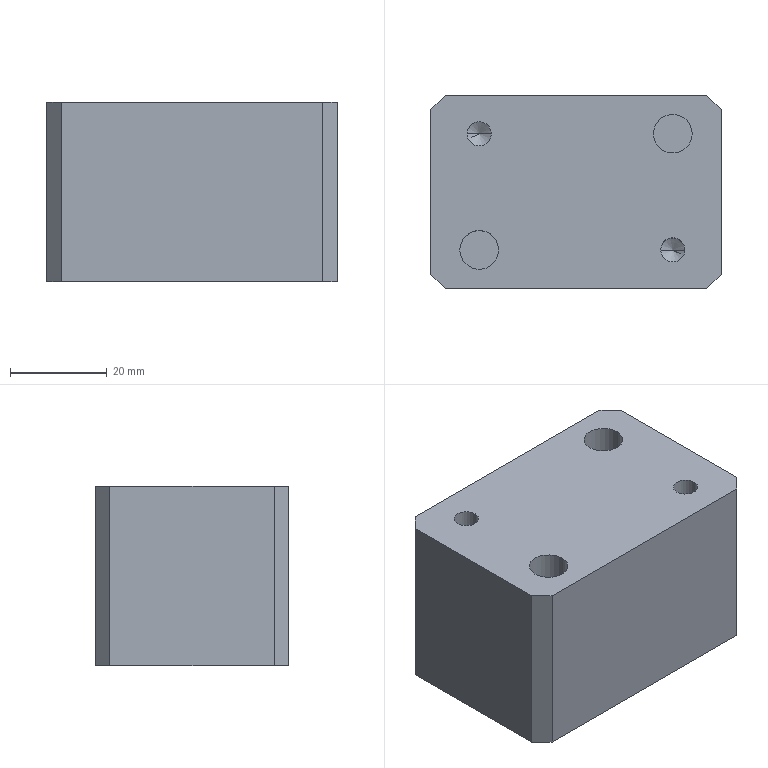Part | SolidWorks | features HoleWzd 4, Chamfer 1, Extrusion 1 | 1 solid | 42 faces | box 60 x 40 x 37 mm | volume 85137 mm3 | cylinder 16 | plane 14 | cone 12 | commonest cylinder face diameters 5 x8 8 x8
STEP:
#1=CARTESIAN_POINT('',(17.998,42.192,0.525));
#2=VERTEX_POINT('',#1);
#3=CARTESIAN_POINT('',(12.998,42.192,0.525));
#4=VERTEX_POINT('',#3);
#5=CARTESIAN_POINT('',(15.498,42.192,0.525));
#6=DIRECTION('',(0.,0.,-1.));
#7=DIRECTION('',(-1.,0.,0.));
#8=AXIS2_PLACEMENT_3D('',#5,#6,#7);
#9=CIRCLE('',#8,2.5);
#10=EDGE_CURVE('',#2,#4,#9,.T.);
#11=ORIENTED_EDGE('',*,*,#10,.F.);
#12=CARTESIAN_POINT('',(18.523,42.192,0.));
#13=VERTEX_POINT('',#12);
#14=CARTESIAN_POINT('',(18.523,42.192,0.));
#15=DIRECTION('',(0.7071,0.,-0.7071));
#16=VECTOR('',#15,1000.);
#17=LINE('',#14,#16);
#18=EDGE_CURVE('',#2,#13,#17,.T.);
#19=ORIENTED_EDGE('',*,*,#18,.T.);
#20=CARTESIAN_POINT('',(12.473,42.192,0.));
#21=VERTEX_POINT('',#20);
#22=CARTESIAN_POINT('',(15.498,42.192,0.));
#23=DIRECTION('',(0.,0.,-1.));
#24=DIRECTION('',(-1.,0.,0.));
#25=AXIS2_PLACEMENT_3D('',#22,#23,#24);
#26=CIRCLE('',#25,3.025);
#27=EDGE_CURVE('',#13,#21,#26,.T.);
#28=ORIENTED_EDGE('',*,*,#27,.T.);
#29=CARTESIAN_POINT('',(12.473,42.192,0.));
#30=DIRECTION('',(-0.7071,0.,-0.7071));
#31=VECTOR('',#30,1000.);
#32=LINE('',#29,#31);
#33=EDGE_CURVE('',#4,#21,#32,.T.);
#34=ORIENTED_EDGE('',*,*,#33,.F.);
#35=EDGE_LOOP('',(#11,#19,#28,#34));
#36=FACE_OUTER_BOUND('',#35,.T.);
#37=CARTESIAN_POINT('',(15.498,42.192,0.));
#38=DIRECTION('',(0.,0.,-1.));
#39=DIRECTION('',(-1.,0.,0.));
#40=AXIS2_PLACEMENT_3D('',#37,#38,#39);
#41=CONICAL_SURFACE('',#40,3.025,0.7854);
#42=ADVANCED_FACE('',(#36),#41,.F.);
#43=CARTESIAN_POINT('',(17.998,42.192,12.));
#44=VERTEX_POINT('',#43);
#45=CARTESIAN_POINT('',(12.998,42.192,12.));
#46=VERTEX_POINT('',#45);
#47=CARTESIAN_POINT('',(15.498,42.192,12.));
#48=DIRECTION('',(0.,0.,-1.));
#49=DIRECTION('',(-1.,0.,0.));
#50=AXIS2_PLACEMENT_3D('',#47,#48,#49);
#51=CIRCLE('',#50,2.5);
#52=EDGE_CURVE('',#44,#46,#51,.T.);
#53=ORIENTED_EDGE('',*,*,#52,.F.);
#54=CARTESIAN_POINT('',(17.998,42.192,0.));
#55=DIRECTION('',(0.,0.,-1.));
#56=VECTOR('',#55,1000.);
#57=LINE('',#54,#56);
#58=EDGE_CURVE('',#44,#2,#57,.T.);
#59=ORIENTED_EDGE('',*,*,#58,.T.);
#60=ORIENTED_EDGE('',*,*,#10,.T.);
#61=CARTESIAN_POINT('',(12.998,42.192,0.));
#62=DIRECTION('',(0.,0.,-1.));
#63=VECTOR('',#62,1000.);
#64=LINE('',#61,#63);
#65=EDGE_CURVE('',#46,#4,#64,.T.);
#66=ORIENTED_EDGE('',*,*,#65,.F.);
#67=EDGE_LOOP('',(#53,#59,#60,#66));
#68=FACE_OUTER_BOUND('',#67,.T.);
#69=CARTESIAN_POINT('',(15.498,42.192,0.));
#70=DIRECTION('',(0.,0.,-1.));
#71=DIRECTION('',(-1.,0.,0.));
#72=AXIS2_PLACEMENT_3D('',#69,#70,#71);
#73=CYLINDRICAL_SURFACE('',#72,2.5);
#74=ADVANCED_FACE('',(#68),#73,.F.);
#75=CARTESIAN_POINT('',(15.498,42.192,13.502));
#76=VERTEX_POINT('',#75);
#77=CARTESIAN_POINT('',(12.998,42.192,12.));
#78=DIRECTION('',(-0.8572,0.,-0.515));
#79=VECTOR('',#78,1000.);
#80=LINE('',#77,#79);
#81=EDGE_CURVE('',#76,#46,#80,.T.);
#82=ORIENTED_EDGE('',*,*,#81,.F.);
#83=CARTESIAN_POINT('',(17.998,42.192,12.));
#84=DIRECTION('',(0.8572,0.,-0.515));
#85=VECTOR('',#84,1000.);
#86=LINE('',#83,#85);
#87=EDGE_CURVE('',#76,#44,#86,.T.);
#88=ORIENTED_EDGE('',*,*,#87,.T.);
#89=ORIENTED_EDGE('',*,*,#52,.T.);
#90=EDGE_LOOP('',(#82,#88,#89));
#91=FACE_OUTER_BOUND('',#90,.T.);
#92=CARTESIAN_POINT('',(15.498,42.192,12.));
#93=DIRECTION('',(0.,0.,-1.));
#94=DIRECTION('',(-1.,0.,0.));
#95=AXIS2_PLACEMENT_3D('',#92,#93,#94);
#96=CONICAL_SURFACE('',#95,2.5,1.03);
#97=ADVANCED_FACE('',(#91),#96,.F.);
#98=CARTESIAN_POINT('',(-22.002,18.192,0.525));
#99=VERTEX_POINT('',#98);
#100=CARTESIAN_POINT('',(-27.002,18.192,0.525));
#101=VERTEX_POINT('',#100);
#102=CARTESIAN_POINT('',(-24.502,18.192,0.525));
#103=DIRECTION('',(0.,0.,-1.));
#104=DIRECTION('',(-1.,0.,0.));
#105=AXIS2_PLACEMENT_3D('',#102,#103,#104);
#106=CIRCLE('',#105,2.5);
#107=EDGE_CURVE('',#99,#101,#106,.T.);
#108=ORIENTED_EDGE('',*,*,#107,.F.);
#109=CARTESIAN_POINT('',(-21.477,18.192,0.));
#110=VERTEX_POINT('',#109);
#111=CARTESIAN_POINT('',(-21.477,18.192,0.));
#112=DIRECTION('',(0.7071,0.,-0.7071));
#113=VECTOR('',#112,1000.);
#114=LINE('',#111,#113);
#115=EDGE_CURVE('',#99,#110,#114,.T.);
#116=ORIENTED_EDGE('',*,*,#115,.T.);
#117=CARTESIAN_POINT('',(-27.527,18.192,0.));
#118=VERTEX_POINT('',#117);
#119=CARTESIAN_POINT('',(-24.502,18.192,0.));
#120=DIRECTION('',(0.,0.,-1.));
#121=DIRECTION('',(-1.,0.,0.));
#122=AXIS2_PLACEMENT_3D('',#119,#120,#121);
#123=CIRCLE('',#122,3.025);
#124=EDGE_CURVE('',#110,#118,#123,.T.);
#125=ORIENTED_EDGE('',*,*,#124,.T.);
#126=CARTESIAN_POINT('',(-27.527,18.192,0.));
#127=DIRECTION('',(-0.7071,0.,-0.7071));
#128=VECTOR('',#127,1000.);
#129=LINE('',#126,#128);
#130=EDGE_CURVE('',#101,#118,#129,.T.);
#131=ORIENTED_EDGE('',*,*,#130,.F.);
#132=EDGE_LOOP('',(#108,#116,#125,#131));
#133=FACE_OUTER_BOUND('',#132,.T.);
#134=CARTESIAN_POINT('',(-24.502,18.192,0.));
#135=DIRECTION('',(0.,0.,-1.));
#136=DIRECTION('',(-1.,0.,0.));
#137=AXIS2_PLACEMENT_3D('',#134,#135,#136);
#138=CONICAL_SURFACE('',#137,3.025,0.7854);
#139=ADVANCED_FACE('',(#133),#138,.F.);
#140=CARTESIAN_POINT('',(-22.002,18.192,12.));
#141=VERTEX_POINT('',#140);
#142=CARTESIAN_POINT('',(-27.002,18.192,12.));
#143=VERTEX_POINT('',#142);
#144=CARTESIAN_POINT('',(-24.502,18.192,12.));
#145=DIRECTION('',(0.,0.,-1.));
#146=DIRECTION('',(-1.,0.,0.));
#147=AXIS2_PLACEMENT_3D('',#144,#145,#146);
#148=CIRCLE('',#147,2.5);
#149=EDGE_CURVE('',#141,#143,#148,.T.);
#150=ORIENTED_EDGE('',*,*,#149,.F.);
#151=CARTESIAN_POINT('',(-22.002,18.192,0.));
#152=DIRECTION('',(0.,0.,-1.));
#153=VECTOR('',#152,1000.);
#154=LINE('',#151,#153);
#155=EDGE_CURVE('',#141,#99,#154,.T.);
#156=ORIENTED_EDGE('',*,*,#155,.T.);
#157=ORIENTED_EDGE('',*,*,#107,.T.);
#158=CARTESIAN_POINT('',(-27.002,18.192,0.));
#159=DIRECTION('',(0.,0.,-1.));
#160=VECTOR('',#159,1000.);
#161=LINE('',#158,#160);
#162=EDGE_CURVE('',#143,#101,#161,.T.);
#163=ORIENTED_EDGE('',*,*,#162,.F.);
#164=EDGE_LOOP('',(#150,#156,#157,#163));
#165=FACE_OUTER_BOUND('',#164,.T.);
#166=CARTESIAN_POINT('',(-24.502,18.192,0.));
#167=DIRECTION('',(0.,0.,-1.));
#168=DIRECTION('',(-1.,0.,0.));
#169=AXIS2_PLACEMENT_3D('',#166,#167,#168);
#170=CYLINDRICAL_SURFACE('',#169,2.5);
#171=ADVANCED_FACE('',(#165),#170,.F.);
#172=CARTESIAN_POINT('',(-24.502,18.192,13.502));
#173=VERTEX_POINT('',#172);
#174=CARTESIAN_POINT('',(-27.002,18.192,12.));
#175=DIRECTION('',(-0.8572,0.,-0.515));
#176=VECTOR('',#175,1000.);
#177=LINE('',#174,#176);
#178=EDGE_CURVE('',#173,#143,#177,.T.);
#179=ORIENTED_EDGE('',*,*,#178,.F.);
#180=CARTESIAN_POINT('',(-22.002,18.192,12.));
#181=DIRECTION('',(0.8572,0.,-0.515));
#182=VECTOR('',#181,1000.);
#183=LINE('',#180,#182);
#184=EDGE_CURVE('',#173,#141,#183,.T.);
#185=ORIENTED_EDGE('',*,*,#184,.T.);
#186=ORIENTED_EDGE('',*,*,#149,.T.);
#187=EDGE_LOOP('',(#179,#185,#186));
#188=FACE_OUTER_BOUND('',#187,.T.);
#189=CARTESIAN_POINT('',(-24.502,18.192,12.));
#190=DIRECTION('',(0.,0.,-1.));
#191=DIRECTION('',(-1.,0.,0.));
#192=AXIS2_PLACEMENT_3D('',#189,#190,#191);
#193=CONICAL_SURFACE('',#192,2.5,1.03);
#194=ADVANCED_FACE('',(#188),#193,.F.);
#195=CARTESIAN_POINT('',(-20.502,42.192,10.));
#196=VERTEX_POINT('',#195);
#197=CARTESIAN_POINT('',(-28.502,42.192,10.));
#198=VERTEX_POINT('',#197);
#199=CARTESIAN_POINT('',(-24.502,42.192,10.));
#200=DIRECTION('',(0.,0.,-1.));
#201=DIRECTION('',(-1.,0.,0.));
#202=AXIS2_PLACEMENT_3D('',#199,#200,#201);
#203=CIRCLE('',#202,4.);
#204=EDGE_CURVE('',#196,#198,#203,.T.);
#205=ORIENTED_EDGE('',*,*,#204,.F.);
#206=CARTESIAN_POINT('',(-20.502,42.192,0.));
#207=VERTEX_POINT('',#206);
#208=CARTESIAN_POINT('',(-20.502,42.192,0.));
#209=DIRECTION('',(0.,0.,-1.));
#210=VECTOR('',#209,1000.);
#211=LINE('',#208,#210);
#212=EDGE_CURVE('',#196,#207,#211,.T.);
#213=ORIENTED_EDGE('',*,*,#212,.T.);
#214=CARTESIAN_POINT('',(-28.502,42.192,0.));
#215=VERTEX_POINT('',#214);
#216=CARTESIAN_POINT('',(-24.502,42.192,0.));
#217=DIRECTION('',(0.,0.,-1.));
#218=DIRECTION('',(-1.,0.,0.));
#219=AXIS2_PLACEMENT_3D('',#216,#217,#218);
#220=CIRCLE('',#219,4.);
#221=EDGE_CURVE('',#207,#215,#220,.T.);
#222=ORIENTED_EDGE('',*,*,#221,.T.);
#223=CARTESIAN_POINT('',(-28.502,42.192,0.));
#224=DIRECTION('',(0.,0.,-1.));
#225=VECTOR('',#224,1000.);
#226=LINE('',#223,#225);
#227=EDGE_CURVE('',#198,#215,#226,.T.);
#228=ORIENTED_EDGE('',*,*,#227,.F.);
#229=EDGE_LOOP('',(#205,#213,#222,#228));
#230=FACE_OUTER_BOUND('',#229,.T.);
#231=CARTESIAN_POINT('',(-24.502,42.192,0.));
#232=DIRECTION('',(0.,0.,-1.));
#233=DIRECTION('',(-1.,0.,0.));
#234=AXIS2_PLACEMENT_3D('',#231,#232,#233);
#235=CYLINDRICAL_SURFACE('',#234,4.);
#236=ADVANCED_FACE('',(#230),#235,.F.);
#237=CARTESIAN_POINT('',(19.498,18.192,10.));
#238=VERTEX_POINT('',#237);
#239=CARTESIAN_POINT('',(11.498,18.192,10.));
#240=VERTEX_POINT('',#239);
#241=CARTESIAN_POINT('',(15.498,18.192,10.));
#242=DIRECTION('',(0.,0.,-1.));
#243=DIRECTION('',(-1.,0.,0.));
#244=AXIS2_PLACEMENT_3D('',#241,#242,#243);
#245=CIRCLE('',#244,4.);
#246=EDGE_CURVE('',#238,#240,#245,.T.);
#247=ORIENTED_EDGE('',*,*,#246,.F.);
#248=CARTESIAN_POINT('',(19.498,18.192,0.));
#249=VERTEX_POINT('',#248);
#250=CARTESIAN_POINT('',(19.498,18.192,0.));
#251=DIRECTION('',(0.,0.,-1.));
#252=VECTOR('',#251,1000.);
#253=LINE('',#250,#252);
#254=EDGE_CURVE('',#238,#249,#253,.T.);
#255=ORIENTED_EDGE('',*,*,#254,.T.);
#256=CARTESIAN_POINT('',(11.498,18.192,0.));
#257=VERTEX_POINT('',#256);
#258=CARTESIAN_POINT('',(15.498,18.192,0.));
#259=DIRECTION('',(0.,0.,-1.));
#260=DIRECTION('',(-1.,0.,0.));
#261=AXIS2_PLACEMENT_3D('',#258,#259,#260);
#262=CIRCLE('',#261,4.);
#263=EDGE_CURVE('',#249,#257,#262,.T.);
#264=ORIENTED_EDGE('',*,*,#263,.T.);
#265=CARTESIAN_POINT('',(11.498,18.192,0.));
#266=DIRECTION('',(0.,0.,-1.));
#267=VECTOR('',#266,1000.);
#268=LINE('',#265,#267);
#269=EDGE_CURVE('',#240,#257,#268,.T.);
#270=ORIENTED_EDGE('',*,*,#269,.F.);
#271=EDGE_LOOP('',(#247,#255,#264,#270));
#272=FACE_OUTER_BOUND('',#271,.T.);
#273=CARTESIAN_POINT('',(15.498,18.192,0.));
#274=DIRECTION('',(0.,0.,-1.));
#275=DIRECTION('',(-1.,0.,0.));
#276=AXIS2_PLACEMENT_3D('',#273,#274,#275);
#277=CYLINDRICAL_SURFACE('',#276,4.);
#278=ADVANCED_FACE('',(#272),#277,.F.);
#279=CARTESIAN_POINT('',(11.498,42.192,27.));
#280=VERTEX_POINT('',#279);
#281=CARTESIAN_POINT('',(19.498,42.192,27.));
#282=VERTEX_POINT('',#281);
#283=CARTESIAN_POINT('',(15.498,42.192,27.));
#284=DIRECTION('',(0.,0.,1.));
#285=DIRECTION('',(1.,0.,0.));
#286=AXIS2_PLACEMENT_3D('',#283,#284,#285);
#287=CIRCLE('',#286,4.);
#288=EDGE_CURVE('',#280,#282,#287,.T.);
#289=ORIENTED_EDGE('',*,*,#288,.F.);
#290=CARTESIAN_POINT('',(11.498,42.192,37.));
#291=VERTEX_POINT('',#290);
#292=CARTESIAN_POINT('',(11.498,42.192,37.));
#293=DIRECTION('',(0.,0.,1.));
#294=VECTOR('',#293,1000.);
#295=LINE('',#292,#294);
#296=EDGE_CURVE('',#280,#291,#295,.T.);
#297=ORIENTED_EDGE('',*,*,#296,.T.);
#298=CARTESIAN_POINT('',(19.498,42.192,37.));
#299=VERTEX_POINT('',#298);
#300=CARTESIAN_POINT('',(15.498,42.192,37.));
#301=DIRECTION('',(0.,0.,1.));
#302=DIRECTION('',(1.,0.,0.));
#303=AXIS2_PLACEMENT_3D('',#300,#301,#302);
#304=CIRCLE('',#303,4.);
#305=EDGE_CURVE('',#291,#299,#304,.T.);
#306=ORIENTED_EDGE('',*,*,#305,.T.);
#307=CARTESIAN_POINT('',(19.498,42.192,37.));
#308=DIRECTION('',(0.,0.,1.));
#309=VECTOR('',#308,1000.);
#310=LINE('',#307,#309);
#311=EDGE_CURVE('',#282,#299,#310,.T.);
#312=ORIENTED_EDGE('',*,*,#311,.F.);
#313=EDGE_LOOP('',(#289,#297,#306,#312));
#314=FACE_OUTER_BOUND('',#313,.T.);
#315=CARTESIAN_POINT('',(15.498,42.192,37.));
#316=DIRECTION('',(0.,0.,1.));
#317=DIRECTION('',(1.,0.,0.));
#318=AXIS2_PLACEMENT_3D('',#315,#316,#317);
#319=CYLINDRICAL_SURFACE('',#318,4.);
#320=ADVANCED_FACE('',(#314),#319,.F.);
#321=CARTESIAN_POINT('',(-28.502,18.192,27.));
#322=VERTEX_POINT('',#321);
#323=CARTESIAN_POINT('',(-20.502,18.192,27.));
#324=VERTEX_POINT('',#323);
#325=CARTESIAN_POINT('',(-24.502,18.192,27.));
#326=DIRECTION('',(0.,0.,1.));
#327=DIRECTION('',(1.,0.,0.));
#328=AXIS2_PLACEMENT_3D('',#325,#326,#327);
#329=CIRCLE('',#328,4.);
#330=EDGE_CURVE('',#322,#324,#329,.T.);
#331=ORIENTED_EDGE('',*,*,#330,.F.);
#332=CARTESIAN_POINT('',(-28.502,18.192,37.));
#333=VERTEX_POINT('',#332);
#334=CARTESIAN_POINT('',(-28.502,18.192,37.));
#335=DIRECTION('',(0.,0.,1.));
#336=VECTOR('',#335,1000.);
#337=LINE('',#334,#336);
#338=EDGE_CURVE('',#322,#333,#337,.T.);
#339=ORIENTED_EDGE('',*,*,#338,.T.);
#340=CARTESIAN_POINT('',(-20.502,18.192,37.));
#341=VERTEX_POINT('',#340);
#342=CARTESIAN_POINT('',(-24.502,18.192,37.));
#343=DIRECTION('',(0.,0.,1.));
#344=DIRECTION('',(1.,0.,0.));
#345=AXIS2_PLACEMENT_3D('',#342,#343,#344);
#346=CIRCLE('',#345,4.);
#347=EDGE_CURVE('',#333,#341,#346,.T.);
#348=ORIENTED_EDGE('',*,*,#347,.T.);
#349=CARTESIAN_POINT('',(-20.502,18.192,37.));
#350=DIRECTION('',(0.,0.,1.));
#351=VECTOR('',#350,1000.);
#352=LINE('',#349,#351);
#353=EDGE_CURVE('',#324,#341,#352,.T.);
#354=ORIENTED_EDGE('',*,*,#353,.F.);
#355=EDGE_LOOP('',(#331,#339,#348,#354));
#356=FACE_OUTER_BOUND('',#355,.T.);
#357=CARTESIAN_POINT('',(-24.502,18.192,37.));
#358=DIRECTION('',(0.,0.,1.));
#359=DIRECTION('',(1.,0.,0.));
#360=AXIS2_PLACEMENT_3D('',#357,#358,#359);
#361=CYLINDRICAL_SURFACE('',#360,4.);
#362=ADVANCED_FACE('',(#356),#361,.F.);
#363=CARTESIAN_POINT('',(-27.002,42.192,25.));
#364=VERTEX_POINT('',#363);
#365=CARTESIAN_POINT('',(-22.002,42.192,25.));
#366=VERTEX_POINT('',#365);
#367=CARTESIAN_POINT('',(-24.502,42.192,25.));
#368=DIRECTION('',(0.,0.,1.));
#369=DIRECTION('',(1.,0.,0.));
#370=AXIS2_PLACEMENT_3D('',#367,#368,#369);
#371=CIRCLE('',#370,2.5);
#372=EDGE_CURVE('',#364,#366,#371,.T.);
#373=ORIENTED_EDGE('',*,*,#372,.F.);
#374=CARTESIAN_POINT('',(-27.002,42.192,37.));
#375=VERTEX_POINT('',#374);
#376=CARTESIAN_POINT('',(-27.002,42.192,37.));
#377=DIRECTION('',(0.,0.,1.));
#378=VECTOR('',#377,1000.);
#379=LINE('',#376,#378);
#380=EDGE_CURVE('',#364,#375,#379,.T.);
#381=ORIENTED_EDGE('',*,*,#380,.T.);
#382=CARTESIAN_POINT('',(-22.002,42.192,37.));
#383=VERTEX_POINT('',#382);
#384=CARTESIAN_POINT('',(-24.502,42.192,37.));
#385=DIRECTION('',(0.,0.,1.));
#386=DIRECTION('',(1.,0.,0.));
#387=AXIS2_PLACEMENT_3D('',#384,#385,#386);
#388=CIRCLE('',#387,2.5);
#389=EDGE_CURVE('',#375,#383,#388,.T.);
#390=ORIENTED_EDGE('',*,*,#389,.T.);
#391=CARTESIAN_POINT('',(-22.002,42.192,37.));
#392=DIRECTION('',(0.,0.,1.));
#393=VECTOR('',#392,1000.);
#394=LINE('',#391,#393);
#395=EDGE_CURVE('',#366,#383,#394,.T.);
#396=ORIENTED_EDGE('',*,*,#395,.F.);
#397=EDGE_LOOP('',(#373,#381,#390,#396));
#398=FACE_OUTER_BOUND('',#397,.T.);
#399=CARTESIAN_POINT('',(-24.502,42.192,37.));
#400=DIRECTION('',(0.,0.,1.));
#401=DIRECTION('',(1.,0.,0.));
#402=AXIS2_PLACEMENT_3D('',#399,#400,#401);
#403=CYLINDRICAL_SURFACE('',#402,2.5);
#404=ADVANCED_FACE('',(#398),#403,.F.);
#405=CARTESIAN_POINT('',(-24.502,42.192,23.498));
#406=VERTEX_POINT('',#405);
#407=CARTESIAN_POINT('',(-22.002,42.192,25.));
#408=DIRECTION('',(0.8572,0.,0.515));
#409=VECTOR('',#408,1000.);
#410=LINE('',#407,#409);
#411=EDGE_CURVE('',#406,#366,#410,.T.);
#412=ORIENTED_EDGE('',*,*,#411,.F.);
#413=CARTESIAN_POINT('',(-27.002,42.192,25.));
#414=DIRECTION('',(-0.8572,0.,0.515));
#415=VECTOR('',#414,1000.);
#416=LINE('',#413,#415);
#417=EDGE_CURVE('',#406,#364,#416,.T.);
#418=ORIENTED_EDGE('',*,*,#417,.T.);
#419=ORIENTED_EDGE('',*,*,#372,.T.);
#420=EDGE_LOOP('',(#412,#418,#419));
#421=FACE_OUTER_BOUND('',#420,.T.);
#422=CARTESIAN_POINT('',(-24.502,42.192,25.));
#423=DIRECTION('',(0.,0.,1.));
#424=DIRECTION('',(1.,0.,0.));
#425=AXIS2_PLACEMENT_3D('',#422,#423,#424);
#426=CONICAL_SURFACE('',#425,2.5,1.03);
#427=ADVANCED_FACE('',(#421),#426,.F.);
#428=CARTESIAN_POINT('',(12.998,18.192,25.));
#429=VERTEX_POINT('',#428);
#430=CARTESIAN_POINT('',(17.998,18.192,25.));
#431=VERTEX_POINT('',#430);
#432=CARTESIAN_POINT('',(15.498,18.192,25.));
#433=DIRECTION('',(0.,0.,1.));
#434=DIRECTION('',(1.,0.,0.));
#435=AXIS2_PLACEMENT_3D('',#432,#433,#434);
#436=CIRCLE('',#435,2.5);
#437=EDGE_CURVE('',#429,#431,#436,.T.);
#438=ORIENTED_EDGE('',*,*,#437,.F.);
#439=CARTESIAN_POINT('',(12.998,18.192,37.));
#440=VERTEX_POINT('',#439);
#441=CARTESIAN_POINT('',(12.998,18.192,37.));
#442=DIRECTION('',(0.,0.,1.));
#443=VECTOR('',#442,1000.);
#444=LINE('',#441,#443);
#445=EDGE_CURVE('',#429,#440,#444,.T.);
#446=ORIENTED_EDGE('',*,*,#445,.T.);
#447=CARTESIAN_POINT('',(17.998,18.192,37.));
#448=VERTEX_POINT('',#447);
#449=CARTESIAN_POINT('',(15.498,18.192,37.));
#450=DIRECTION('',(0.,0.,1.));
#451=DIRECTION('',(1.,0.,0.));
#452=AXIS2_PLACEMENT_3D('',#449,#450,#451);
#453=CIRCLE('',#452,2.5);
#454=EDGE_CURVE('',#440,#448,#453,.T.);
#455=ORIENTED_EDGE('',*,*,#454,.T.);
#456=CARTESIAN_POINT('',(17.998,18.192,37.));
#457=DIRECTION('',(0.,0.,1.));
#458=VECTOR('',#457,1000.);
#459=LINE('',#456,#458);
#460=EDGE_CURVE('',#431,#448,#459,.T.);
#461=ORIENTED_EDGE('',*,*,#460,.F.);
#462=EDGE_LOOP('',(#438,#446,#455,#461));
#463=FACE_OUTER_BOUND('',#462,.T.);
#464=CARTESIAN_POINT('',(15.498,18.192,37.));
#465=DIRECTION('',(0.,0.,1.));
#466=DIRECTION('',(1.,0.,0.));
#467=AXIS2_PLACEMENT_3D('',#464,#465,#466);
#468=CYLINDRICAL_SURFACE('',#467,2.5);
#469=ADVANCED_FACE('',(#463),#468,.F.);
#470=CARTESIAN_POINT('',(15.498,18.192,23.498));
#471=VERTEX_POINT('',#470);
#472=CARTESIAN_POINT('',(17.998,18.192,25.));
#473=DIRECTION('',(0.8572,0.,0.515));
#474=VECTOR('',#473,1000.);
#475=LINE('',#472,#474);
#476=EDGE_CURVE('',#471,#431,#475,.T.);
#477=ORIENTED_EDGE('',*,*,#476,.F.);
#478=CARTESIAN_POINT('',(12.998,18.192,25.));
#479=DIRECTION('',(-0.8572,0.,0.515));
#480=VECTOR('',#479,1000.);
#481=LINE('',#478,#480);
#482=EDGE_CURVE('',#471,#429,#481,.T.);
#483=ORIENTED_EDGE('',*,*,#482,.T.);
#484=ORIENTED_EDGE('',*,*,#437,.T.);
#485=EDGE_LOOP('',(#477,#483,#484));
#486=FACE_OUTER_BOUND('',#485,.T.);
#487=CARTESIAN_POINT('',(15.498,18.192,25.));
#488=DIRECTION('',(0.,0.,1.));
#489=DIRECTION('',(1.,0.,0.));
#490=AXIS2_PLACEMENT_3D('',#487,#488,#489);
#491=CONICAL_SURFACE('',#490,2.5,1.03);
#492=ADVANCED_FACE('',(#486),#491,.F.);
#493=CARTESIAN_POINT('',(-34.502,47.192,0.));
#494=VERTEX_POINT('',#493);
#495=CARTESIAN_POINT('',(-34.502,13.192,0.));
#496=VERTEX_POINT('',#495);
#497=CARTESIAN_POINT('',(-34.502,50.192,0.));
#498=DIRECTION('',(0.,-1.,0.));
#499=VECTOR('',#498,1000.);
#500=LINE('',#497,#499);
#501=EDGE_CURVE('',#494,#496,#500,.T.);
#502=ORIENTED_EDGE('',*,*,#501,.T.);
#503=CARTESIAN_POINT('',(-34.502,13.192,37.));
#504=VERTEX_POINT('',#503);
#505=CARTESIAN_POINT('',(-34.502,13.192,37.));
#506=DIRECTION('',(0.,0.,1.));
#507=VECTOR('',#506,1000.);
#508=LINE('',#505,#507);
#509=EDGE_CURVE('',#496,#504,#508,.T.);
#510=ORIENTED_EDGE('',*,*,#509,.T.);
#511=CARTESIAN_POINT('',(-34.502,47.192,37.));
#512=VERTEX_POINT('',#511);
#513=CARTESIAN_POINT('',(-34.502,50.192,37.));
#514=DIRECTION('',(0.,-1.,0.));
#515=VECTOR('',#514,1000.);
#516=LINE('',#513,#515);
#517=EDGE_CURVE('',#512,#504,#516,.T.);
#518=ORIENTED_EDGE('',*,*,#517,.F.);
#519=CARTESIAN_POINT('',(-34.502,47.192,37.));
#520=DIRECTION('',(0.,0.,-1.));
#521=VECTOR('',#520,1000.);
#522=LINE('',#519,#521);
#523=EDGE_CURVE('',#512,#494,#522,.T.);
#524=ORIENTED_EDGE('',*,*,#523,.T.);
#525=EDGE_LOOP('',(#502,#510,#518,#524));
#526=FACE_OUTER_BOUND('',#525,.T.);
#527=CARTESIAN_POINT('',(-34.502,50.192,37.));
#528=DIRECTION('',(1.,0.,0.));
#529=DIRECTION('',(0.,1.,0.));
#530=AXIS2_PLACEMENT_3D('',#527,#528,#529);
#531=PLANE('',#530);
#532=ADVANCED_FACE('',(#526),#531,.F.);
#533=CARTESIAN_POINT('',(-31.502,10.192,0.));
#534=VERTEX_POINT('',#533);
#535=CARTESIAN_POINT('',(22.498,10.192,0.));
#536=VERTEX_POINT('',#535);
#537=CARTESIAN_POINT('',(-34.502,10.192,0.));
#538=DIRECTION('',(1.,0.,0.));
#539=VECTOR('',#538,1000.);
#540=LINE('',#537,#539);
#541=EDGE_CURVE('',#534,#536,#540,.T.);
#542=ORIENTED_EDGE('',*,*,#541,.T.);
#543=CARTESIAN_POINT('',(22.498,10.192,37.));
#544=VERTEX_POINT('',#543);
#545=CARTESIAN_POINT('',(22.498,10.192,37.));
#546=DIRECTION('',(0.,0.,1.));
#547=VECTOR('',#546,1000.);
#548=LINE('',#545,#547);
#549=EDGE_CURVE('',#536,#544,#548,.T.);
#550=ORIENTED_EDGE('',*,*,#549,.T.);
#551=CARTESIAN_POINT('',(-31.502,10.192,37.));
#552=VERTEX_POINT('',#551);
#553=CARTESIAN_POINT('',(-34.502,10.192,37.));
#554=DIRECTION('',(1.,0.,0.));
#555=VECTOR('',#554,1000.);
#556=LINE('',#553,#555);
#557=EDGE_CURVE('',#552,#544,#556,.T.);
#558=ORIENTED_EDGE('',*,*,#557,.F.);
#559=CARTESIAN_POINT('',(-31.502,10.192,37.));
#560=DIRECTION('',(0.,0.,-1.));
#561=VECTOR('',#560,1000.);
#562=LINE('',#559,#561);
#563=EDGE_CURVE('',#552,#534,#562,.T.);
#564=ORIENTED_EDGE('',*,*,#563,.T.);
#565=EDGE_LOOP('',(#542,#550,#558,#564));
#566=FACE_OUTER_BOUND('',#565,.T.);
#567=CARTESIAN_POINT('',(-34.502,10.192,37.));
#568=DIRECTION('',(0.,1.,0.));
#569=DIRECTION('',(0.,0.,1.));
#570=AXIS2_PLACEMENT_3D('',#567,#568,#569);
#571=PLANE('',#570);
#572=ADVANCED_FACE('',(#566),#571,.F.);
#573=CARTESIAN_POINT('',(25.498,13.192,37.));
#574=VERTEX_POINT('',#573);
#575=CARTESIAN_POINT('',(25.498,47.192,37.));
#576=VERTEX_POINT('',#575);
#577=CARTESIAN_POINT('',(25.498,50.192,37.));
#578=DIRECTION('',(0.,1.,0.));
#579=VECTOR('',#578,1000.);
#580=LINE('',#577,#579);
#581=EDGE_CURVE('',#574,#576,#580,.T.);
#582=ORIENTED_EDGE('',*,*,#581,.F.);
#583=CARTESIAN_POINT('',(25.498,13.192,0.));
#584=VERTEX_POINT('',#583);
#585=CARTESIAN_POINT('',(25.498,13.192,37.));
#586=DIRECTION('',(0.,0.,-1.));
#587=VECTOR('',#586,1000.);
#588=LINE('',#585,#587);
#589=EDGE_CURVE('',#574,#584,#588,.T.);
#590=ORIENTED_EDGE('',*,*,#589,.T.);
#591=CARTESIAN_POINT('',(25.498,47.192,0.));
#592=VERTEX_POINT('',#591);
#593=CARTESIAN_POINT('',(25.498,50.192,0.));
#594=DIRECTION('',(0.,1.,0.));
#595=VECTOR('',#594,1000.);
#596=LINE('',#593,#595);
#597=EDGE_CURVE('',#584,#592,#596,.T.);
#598=ORIENTED_EDGE('',*,*,#597,.T.);
#599=CARTESIAN_POINT('',(25.498,47.192,37.));
#600=DIRECTION('',(0.,0.,1.));
#601=VECTOR('',#600,1000.);
#602=LINE('',#599,#601);
#603=EDGE_CURVE('',#592,#576,#602,.T.);
#604=ORIENTED_EDGE('',*,*,#603,.T.);
#605=EDGE_LOOP('',(#582,#590,#598,#604));
#606=FACE_OUTER_BOUND('',#605,.T.);
#607=CARTESIAN_POINT('',(25.498,50.192,37.));
#608=DIRECTION('',(-1.,0.,0.));
#609=DIRECTION('',(0.,0.,1.));
#610=AXIS2_PLACEMENT_3D('',#607,#608,#609);
#611=PLANE('',#610);
#612=ADVANCED_FACE('',(#606),#611,.F.);
#613=CARTESIAN_POINT('',(22.498,50.192,37.));
#614=VERTEX_POINT('',#613);
#615=CARTESIAN_POINT('',(-31.502,50.192,37.));
#616=VERTEX_POINT('',#615);
#617=CARTESIAN_POINT('',(-34.502,50.192,37.));
#618=DIRECTION('',(-1.,0.,0.));
#619=VECTOR('',#618,1000.);
#620=LINE('',#617,#619);
#621=EDGE_CURVE('',#614,#616,#620,.T.);
#622=ORIENTED_EDGE('',*,*,#621,.F.);
#623=CARTESIAN_POINT('',(22.498,50.192,0.));
#624=VERTEX_POINT('',#623);
#625=CARTESIAN_POINT('',(22.498,50.192,37.));
#626=DIRECTION('',(0.,0.,-1.));
#627=VECTOR('',#626,1000.);
#628=LINE('',#625,#627);
#629=EDGE_CURVE('',#614,#624,#628,.T.);
#630=ORIENTED_EDGE('',*,*,#629,.T.);
#631=CARTESIAN_POINT('',(-31.502,50.192,0.));
#632=VERTEX_POINT('',#631);
#633=CARTESIAN_POINT('',(-34.502,50.192,0.));
#634=DIRECTION('',(-1.,0.,0.));
#635=VECTOR('',#634,1000.);
#636=LINE('',#633,#635);
#637=EDGE_CURVE('',#624,#632,#636,.T.);
#638=ORIENTED_EDGE('',*,*,#637,.T.);
#639=CARTESIAN_POINT('',(-31.502,50.192,37.));
#640=DIRECTION('',(0.,0.,1.));
#641=VECTOR('',#640,1000.);
#642=LINE('',#639,#641);
#643=EDGE_CURVE('',#632,#616,#642,.T.);
#644=ORIENTED_EDGE('',*,*,#643,.T.);
#645=EDGE_LOOP('',(#622,#630,#638,#644));
#646=FACE_OUTER_BOUND('',#645,.T.);
#647=CARTESIAN_POINT('',(-34.502,50.192,37.));
#648=DIRECTION('',(0.,-1.,0.));
#649=DIRECTION('',(0.,0.,-1.));
#650=AXIS2_PLACEMENT_3D('',#647,#648,#649);
#651=PLANE('',#650);
#652=ADVANCED_FACE('',(#646),#651,.F.);
#653=CARTESIAN_POINT('',(15.498,42.192,37.));
#654=DIRECTION('',(0.,0.,1.));
#655=DIRECTION('',(1.,0.,0.));
#656=AXIS2_PLACEMENT_3D('',#653,#654,#655);
#657=CIRCLE('',#656,4.);
#658=EDGE_CURVE('',#299,#291,#657,.T.);
#659=ORIENTED_EDGE('',*,*,#658,.F.);
#660=ORIENTED_EDGE('',*,*,#305,.F.);
#661=EDGE_LOOP('',(#659,#660));
#662=FACE_BOUND('',#661,.T.);
#663=CARTESIAN_POINT('',(-24.502,18.192,37.));
#664=DIRECTION('',(0.,0.,1.));
#665=DIRECTION('',(1.,0.,0.));
#666=AXIS2_PLACEMENT_3D('',#663,#664,#665);
#667=CIRCLE('',#666,4.);
#668=EDGE_CURVE('',#341,#333,#667,.T.);
#669=ORIENTED_EDGE('',*,*,#668,.F.);
#670=ORIENTED_EDGE('',*,*,#347,.F.);
#671=EDGE_LOOP('',(#669,#670));
#672=FACE_BOUND('',#671,.T.);
#673=CARTESIAN_POINT('',(-24.502,42.192,37.));
#674=DIRECTION('',(0.,0.,1.));
#675=DIRECTION('',(1.,0.,0.));
#676=AXIS2_PLACEMENT_3D('',#673,#674,#675);
#677=CIRCLE('',#676,2.5);
#678=EDGE_CURVE('',#383,#375,#677,.T.);
#679=ORIENTED_EDGE('',*,*,#678,.F.);
#680=ORIENTED_EDGE('',*,*,#389,.F.);
#681=EDGE_LOOP('',(#679,#680));
#682=FACE_BOUND('',#681,.T.);
#683=CARTESIAN_POINT('',(15.498,18.192,37.));
#684=DIRECTION('',(0.,0.,1.));
#685=DIRECTION('',(1.,0.,0.));
#686=AXIS2_PLACEMENT_3D('',#683,#684,#685);
#687=CIRCLE('',#686,2.5);
#688=EDGE_CURVE('',#448,#440,#687,.T.);
#689=ORIENTED_EDGE('',*,*,#688,.F.);
#690=ORIENTED_EDGE('',*,*,#454,.F.);
#691=EDGE_LOOP('',(#689,#690));
#692=FACE_BOUND('',#691,.T.);
#693=ORIENTED_EDGE('',*,*,#557,.T.);
#694=CARTESIAN_POINT('',(6.153,-6.153,37.));
#695=DIRECTION('',(0.7071,0.7071,0.));
#696=VECTOR('',#695,1000.);
#697=LINE('',#694,#696);
#698=EDGE_CURVE('',#544,#574,#697,.T.);
#699=ORIENTED_EDGE('',*,*,#698,.T.);
#700=ORIENTED_EDGE('',*,*,#581,.T.);
#701=CARTESIAN_POINT('',(36.345,36.345,37.));
#702=DIRECTION('',(-0.7071,0.7071,0.));
#703=VECTOR('',#702,1000.);
#704=LINE('',#701,#703);
#705=EDGE_CURVE('',#576,#614,#704,.T.);
#706=ORIENTED_EDGE('',*,*,#705,.T.);
#707=ORIENTED_EDGE('',*,*,#621,.T.);
#708=CARTESIAN_POINT('',(-40.847,40.847,37.));
#709=DIRECTION('',(-0.7071,-0.7071,0.));
#710=VECTOR('',#709,1000.);
#711=LINE('',#708,#710);
#712=EDGE_CURVE('',#616,#512,#711,.T.);
#713=ORIENTED_EDGE('',*,*,#712,.T.);
#714=ORIENTED_EDGE('',*,*,#517,.T.);
#715=CARTESIAN_POINT('',(-10.655,-10.655,37.));
#716=DIRECTION('',(0.7071,-0.7071,0.));
#717=VECTOR('',#716,1000.);
#718=LINE('',#715,#717);
#719=EDGE_CURVE('',#504,#552,#718,.T.);
#720=ORIENTED_EDGE('',*,*,#719,.T.);
#721=EDGE_LOOP('',(#693,#699,#700,#706,#707,#713,#714,#720));
#722=FACE_OUTER_BOUND('',#721,.T.);
#723=CARTESIAN_POINT('',(0.,0.,37.));
#724=DIRECTION('',(0.,0.,1.));
#725=DIRECTION('',(1.,0.,0.));
#726=AXIS2_PLACEMENT_3D('',#723,#724,#725);
#727=PLANE('',#726);
#728=ADVANCED_FACE('',(#662,#672,#682,#692,#722),#727,.T.);
#729=CARTESIAN_POINT('',(15.498,42.192,0.));
#730=DIRECTION('',(0.,0.,-1.));
#731=DIRECTION('',(-1.,0.,0.));
#732=AXIS2_PLACEMENT_3D('',#729,#730,#731);
#733=CIRCLE('',#732,3.025);
#734=EDGE_CURVE('',#21,#13,#733,.T.);
#735=ORIENTED_EDGE('',*,*,#734,.F.);
#736=ORIENTED_EDGE('',*,*,#27,.F.);
#737=EDGE_LOOP('',(#735,#736));
#738=FACE_BOUND('',#737,.T.);
#739=CARTESIAN_POINT('',(-24.502,18.192,0.));
#740=DIRECTION('',(0.,0.,-1.));
#741=DIRECTION('',(-1.,0.,0.));
#742=AXIS2_PLACEMENT_3D('',#739,#740,#741);
#743=CIRCLE('',#742,3.025);
#744=EDGE_CURVE('',#118,#110,#743,.T.);
#745=ORIENTED_EDGE('',*,*,#744,.F.);
#746=ORIENTED_EDGE('',*,*,#124,.F.);
#747=EDGE_LOOP('',(#745,#746));
#748=FACE_BOUND('',#747,.T.);
#749=CARTESIAN_POINT('',(-24.502,42.192,0.));
#750=DIRECTION('',(0.,0.,-1.));
#751=DIRECTION('',(-1.,0.,0.));
#752=AXIS2_PLACEMENT_3D('',#749,#750,#751);
#753=CIRCLE('',#752,4.);
#754=EDGE_CURVE('',#215,#207,#753,.T.);
#755=ORIENTED_EDGE('',*,*,#754,.F.);
#756=ORIENTED_EDGE('',*,*,#221,.F.);
#757=EDGE_LOOP('',(#755,#756));
#758=FACE_BOUND('',#757,.T.);
#759=CARTESIAN_POINT('',(15.498,18.192,0.));
#760=DIRECTION('',(0.,0.,-1.));
#761=DIRECTION('',(-1.,0.,0.));
#762=AXIS2_PLACEMENT_3D('',#759,#760,#761);
#763=CIRCLE('',#762,4.);
#764=EDGE_CURVE('',#257,#249,#763,.T.);
#765=ORIENTED_EDGE('',*,*,#764,.F.);
#766=ORIENTED_EDGE('',*,*,#263,.F.);
#767=EDGE_LOOP('',(#765,#766));
#768=FACE_BOUND('',#767,.T.);
#769=ORIENTED_EDGE('',*,*,#597,.F.);
#770=CARTESIAN_POINT('',(25.498,13.192,0.));
#771=DIRECTION('',(-0.7071,-0.7071,0.));
#772=VECTOR('',#771,1000.);
#773=LINE('',#770,#772);
#774=EDGE_CURVE('',#584,#536,#773,.T.);
#775=ORIENTED_EDGE('',*,*,#774,.T.);
#776=ORIENTED_EDGE('',*,*,#541,.F.);
#777=CARTESIAN_POINT('',(-31.502,10.192,0.));
#778=DIRECTION('',(-0.7071,0.7071,0.));
#779=VECTOR('',#778,1000.);
#780=LINE('',#777,#779);
#781=EDGE_CURVE('',#534,#496,#780,.T.);
#782=ORIENTED_EDGE('',*,*,#781,.T.);
#783=ORIENTED_EDGE('',*,*,#501,.F.);
#784=CARTESIAN_POINT('',(-34.502,47.192,0.));
#785=DIRECTION('',(0.7071,0.7071,0.));
#786=VECTOR('',#785,1000.);
#787=LINE('',#784,#786);
#788=EDGE_CURVE('',#494,#632,#787,.T.);
#789=ORIENTED_EDGE('',*,*,#788,.T.);
#790=ORIENTED_EDGE('',*,*,#637,.F.);
#791=CARTESIAN_POINT('',(22.498,50.192,0.));
#792=DIRECTION('',(0.7071,-0.7071,0.));
#793=VECTOR('',#792,1000.);
#794=LINE('',#791,#793);
#795=EDGE_CURVE('',#624,#592,#794,.T.);
#796=ORIENTED_EDGE('',*,*,#795,.T.);
#797=EDGE_LOOP('',(#769,#775,#776,#782,#783,#789,#790,#796));
#798=FACE_OUTER_BOUND('',#797,.T.);
#799=CARTESIAN_POINT('',(0.,0.,0.));
#800=DIRECTION('',(0.,0.,1.));
#801=DIRECTION('',(1.,0.,0.));
#802=AXIS2_PLACEMENT_3D('',#799,#800,#801);
#803=PLANE('',#802);
#804=ADVANCED_FACE('',(#738,#748,#758,#768,#798),#803,.F.);
#805=ORIENTED_EDGE('',*,*,#698,.F.);
#806=ORIENTED_EDGE('',*,*,#549,.F.);
#807=ORIENTED_EDGE('',*,*,#774,.F.);
#808=ORIENTED_EDGE('',*,*,#589,.F.);
#809=EDGE_LOOP('',(#805,#806,#807,#808));
#810=FACE_OUTER_BOUND('',#809,.T.);
#811=CARTESIAN_POINT('',(25.498,13.192,37.));
#812=DIRECTION('',(-0.7071,0.7071,0.));
#813=DIRECTION('',(0.,0.,-1.));
#814=AXIS2_PLACEMENT_3D('',#811,#812,#813);
#815=PLANE('',#814);
#816=ADVANCED_FACE('',(#810),#815,.F.);
#817=ORIENTED_EDGE('',*,*,#705,.F.);
#818=ORIENTED_EDGE('',*,*,#603,.F.);
#819=ORIENTED_EDGE('',*,*,#795,.F.);
#820=ORIENTED_EDGE('',*,*,#629,.F.);
#821=EDGE_LOOP('',(#817,#818,#819,#820));
#822=FACE_OUTER_BOUND('',#821,.T.);
#823=CARTESIAN_POINT('',(22.498,50.192,37.));
#824=DIRECTION('',(-0.7071,-0.7071,0.));
#825=DIRECTION('',(0.,0.,-1.));
#826=AXIS2_PLACEMENT_3D('',#823,#824,#825);
#827=PLANE('',#826);
#828=ADVANCED_FACE('',(#822),#827,.F.);
#829=ORIENTED_EDGE('',*,*,#719,.F.);
#830=ORIENTED_EDGE('',*,*,#509,.F.);
#831=ORIENTED_EDGE('',*,*,#781,.F.);
#832=ORIENTED_EDGE('',*,*,#563,.F.);
#833=EDGE_LOOP('',(#829,#830,#831,#832));
#834=FACE_OUTER_BOUND('',#833,.T.);
#835=CARTESIAN_POINT('',(-31.502,10.192,37.));
#836=DIRECTION('',(0.7071,0.7071,0.));
#837=DIRECTION('',(0.,0.,-1.));
#838=AXIS2_PLACEMENT_3D('',#835,#836,#837);
#839=PLANE('',#838);
#840=ADVANCED_FACE('',(#834),#839,.F.);
#841=ORIENTED_EDGE('',*,*,#712,.F.);
#842=ORIENTED_EDGE('',*,*,#643,.F.);
#843=ORIENTED_EDGE('',*,*,#788,.F.);
#844=ORIENTED_EDGE('',*,*,#523,.F.);
#845=EDGE_LOOP('',(#841,#842,#843,#844));
#846=FACE_OUTER_BOUND('',#845,.T.);
#847=CARTESIAN_POINT('',(-34.502,47.192,37.));
#848=DIRECTION('',(0.7071,-0.7071,0.));
#849=DIRECTION('',(0.,0.,-1.));
#850=AXIS2_PLACEMENT_3D('',#847,#848,#849);
#851=PLANE('',#850);
#852=ADVANCED_FACE('',(#846),#851,.F.);
#853=ORIENTED_EDGE('',*,*,#482,.F.);
#854=ORIENTED_EDGE('',*,*,#476,.T.);
#855=CARTESIAN_POINT('',(15.498,18.192,25.));
#856=DIRECTION('',(0.,0.,1.));
#857=DIRECTION('',(1.,0.,0.));
#858=AXIS2_PLACEMENT_3D('',#855,#856,#857);
#859=CIRCLE('',#858,2.5);
#860=EDGE_CURVE('',#431,#429,#859,.T.);
#861=ORIENTED_EDGE('',*,*,#860,.T.);
#862=EDGE_LOOP('',(#853,#854,#861));
#863=FACE_OUTER_BOUND('',#862,.T.);
#864=CARTESIAN_POINT('',(15.498,18.192,25.));
#865=DIRECTION('',(0.,0.,1.));
#866=DIRECTION('',(1.,0.,0.));
#867=AXIS2_PLACEMENT_3D('',#864,#865,#866);
#868=CONICAL_SURFACE('',#867,2.5,1.03);
#869=ADVANCED_FACE('',(#863),#868,.F.);
#870=ORIENTED_EDGE('',*,*,#445,.F.);
#871=ORIENTED_EDGE('',*,*,#860,.F.);
#872=ORIENTED_EDGE('',*,*,#460,.T.);
#873=ORIENTED_EDGE('',*,*,#688,.T.);
#874=EDGE_LOOP('',(#870,#871,#872,#873));
#875=FACE_OUTER_BOUND('',#874,.T.);
#876=CARTESIAN_POINT('',(15.498,18.192,37.));
#877=DIRECTION('',(0.,0.,1.));
#878=DIRECTION('',(1.,0.,0.));
#879=AXIS2_PLACEMENT_3D('',#876,#877,#878);
#880=CYLINDRICAL_SURFACE('',#879,2.5);
#881=ADVANCED_FACE('',(#875),#880,.F.);
#882=ORIENTED_EDGE('',*,*,#417,.F.);
#883=ORIENTED_EDGE('',*,*,#411,.T.);
#884=CARTESIAN_POINT('',(-24.502,42.192,25.));
#885=DIRECTION('',(0.,0.,1.));
#886=DIRECTION('',(1.,0.,0.));
#887=AXIS2_PLACEMENT_3D('',#884,#885,#886);
#888=CIRCLE('',#887,2.5);
#889=EDGE_CURVE('',#366,#364,#888,.T.);
#890=ORIENTED_EDGE('',*,*,#889,.T.);
#891=EDGE_LOOP('',(#882,#883,#890));
#892=FACE_OUTER_BOUND('',#891,.T.);
#893=CARTESIAN_POINT('',(-24.502,42.192,25.));
#894=DIRECTION('',(0.,0.,1.));
#895=DIRECTION('',(1.,0.,0.));
#896=AXIS2_PLACEMENT_3D('',#893,#894,#895);
#897=CONICAL_SURFACE('',#896,2.5,1.03);
#898=ADVANCED_FACE('',(#892),#897,.F.);
#899=ORIENTED_EDGE('',*,*,#380,.F.);
#900=ORIENTED_EDGE('',*,*,#889,.F.);
#901=ORIENTED_EDGE('',*,*,#395,.T.);
#902=ORIENTED_EDGE('',*,*,#678,.T.);
#903=EDGE_LOOP('',(#899,#900,#901,#902));
#904=FACE_OUTER_BOUND('',#903,.T.);
#905=CARTESIAN_POINT('',(-24.502,42.192,37.));
#906=DIRECTION('',(0.,0.,1.));
#907=DIRECTION('',(1.,0.,0.));
#908=AXIS2_PLACEMENT_3D('',#905,#906,#907);
#909=CYLINDRICAL_SURFACE('',#908,2.5);
#910=ADVANCED_FACE('',(#904),#909,.F.);
#911=CARTESIAN_POINT('',(-24.502,18.192,27.));
#912=DIRECTION('',(0.,0.,1.));
#913=DIRECTION('',(1.,0.,0.));
#914=AXIS2_PLACEMENT_3D('',#911,#912,#913);
#915=CIRCLE('',#914,4.);
#916=EDGE_CURVE('',#324,#322,#915,.T.);
#917=ORIENTED_EDGE('',*,*,#916,.T.);
#918=ORIENTED_EDGE('',*,*,#330,.T.);
#919=EDGE_LOOP('',(#917,#918));
#920=FACE_OUTER_BOUND('',#919,.T.);
#921=CARTESIAN_POINT('',(-24.502,18.192,27.));
#922=DIRECTION('',(0.,0.,-1.));
#923=DIRECTION('',(-1.,0.,0.));
#924=AXIS2_PLACEMENT_3D('',#921,#922,#923);
#925=PLANE('',#924);
#926=ADVANCED_FACE('',(#920),#925,.F.);
#927=ORIENTED_EDGE('',*,*,#338,.F.);
#928=ORIENTED_EDGE('',*,*,#916,.F.);
#929=ORIENTED_EDGE('',*,*,#353,.T.);
#930=ORIENTED_EDGE('',*,*,#668,.T.);
#931=EDGE_LOOP('',(#927,#928,#929,#930));
#932=FACE_OUTER_BOUND('',#931,.T.);
#933=CARTESIAN_POINT('',(-24.502,18.192,37.));
#934=DIRECTION('',(0.,0.,1.));
#935=DIRECTION('',(1.,0.,0.));
#936=AXIS2_PLACEMENT_3D('',#933,#934,#935);
#937=CYLINDRICAL_SURFACE('',#936,4.);
#938=ADVANCED_FACE('',(#932),#937,.F.);
#939=CARTESIAN_POINT('',(15.498,42.192,27.));
#940=DIRECTION('',(0.,0.,1.));
#941=DIRECTION('',(1.,0.,0.));
#942=AXIS2_PLACEMENT_3D('',#939,#940,#941);
#943=CIRCLE('',#942,4.);
#944=EDGE_CURVE('',#282,#280,#943,.T.);
#945=ORIENTED_EDGE('',*,*,#944,.T.);
#946=ORIENTED_EDGE('',*,*,#288,.T.);
#947=EDGE_LOOP('',(#945,#946));
#948=FACE_OUTER_BOUND('',#947,.T.);
#949=CARTESIAN_POINT('',(15.498,42.192,27.));
#950=DIRECTION('',(0.,0.,-1.));
#951=DIRECTION('',(-1.,0.,0.));
#952=AXIS2_PLACEMENT_3D('',#949,#950,#951);
#953=PLANE('',#952);
#954=ADVANCED_FACE('',(#948),#953,.F.);
#955=ORIENTED_EDGE('',*,*,#296,.F.);
#956=ORIENTED_EDGE('',*,*,#944,.F.);
#957=ORIENTED_EDGE('',*,*,#311,.T.);
#958=ORIENTED_EDGE('',*,*,#658,.T.);
#959=EDGE_LOOP('',(#955,#956,#957,#958));
#960=FACE_OUTER_BOUND('',#959,.T.);
#961=CARTESIAN_POINT('',(15.498,42.192,37.));
#962=DIRECTION('',(0.,0.,1.));
#963=DIRECTION('',(1.,0.,0.));
#964=AXIS2_PLACEMENT_3D('',#961,#962,#963);
#965=CYLINDRICAL_SURFACE('',#964,4.);
#966=ADVANCED_FACE('',(#960),#965,.F.);
#967=CARTESIAN_POINT('',(15.498,18.192,10.));
#968=DIRECTION('',(0.,0.,-1.));
#969=DIRECTION('',(-1.,0.,0.));
#970=AXIS2_PLACEMENT_3D('',#967,#968,#969);
#971=CIRCLE('',#970,4.);
#972=EDGE_CURVE('',#240,#238,#971,.T.);
#973=ORIENTED_EDGE('',*,*,#972,.T.);
#974=ORIENTED_EDGE('',*,*,#246,.T.);
#975=EDGE_LOOP('',(#973,#974));
#976=FACE_OUTER_BOUND('',#975,.T.);
#977=CARTESIAN_POINT('',(15.498,18.192,10.));
#978=DIRECTION('',(0.,0.,1.));
#979=DIRECTION('',(1.,0.,0.));
#980=AXIS2_PLACEMENT_3D('',#977,#978,#979);
#981=PLANE('',#980);
#982=ADVANCED_FACE('',(#976),#981,.F.);
#983=ORIENTED_EDGE('',*,*,#254,.F.);
#984=ORIENTED_EDGE('',*,*,#972,.F.);
#985=ORIENTED_EDGE('',*,*,#269,.T.);
#986=ORIENTED_EDGE('',*,*,#764,.T.);
#987=EDGE_LOOP('',(#983,#984,#985,#986));
#988=FACE_OUTER_BOUND('',#987,.T.);
#989=CARTESIAN_POINT('',(15.498,18.192,0.));
#990=DIRECTION('',(0.,0.,-1.));
#991=DIRECTION('',(-1.,0.,0.));
#992=AXIS2_PLACEMENT_3D('',#989,#990,#991);
#993=CYLINDRICAL_SURFACE('',#992,4.);
#994=ADVANCED_FACE('',(#988),#993,.F.);
#995=CARTESIAN_POINT('',(-24.502,42.192,10.));
#996=DIRECTION('',(0.,0.,-1.));
#997=DIRECTION('',(-1.,0.,0.));
#998=AXIS2_PLACEMENT_3D('',#995,#996,#997);
#999=CIRCLE('',#998,4.);
#1000=EDGE_CURVE('',#198,#196,#999,.T.);
#1001=ORIENTED_EDGE('',*,*,#1000,.T.);
#1002=ORIENTED_EDGE('',*,*,#204,.T.);
#1003=EDGE_LOOP('',(#1001,#1002));
#1004=FACE_OUTER_BOUND('',#1003,.T.);
#1005=CARTESIAN_POINT('',(-24.502,42.192,10.));
#1006=DIRECTION('',(0.,0.,1.));
#1007=DIRECTION('',(1.,0.,0.));
#1008=AXIS2_PLACEMENT_3D('',#1005,#1006,#1007);
#1009=PLANE('',#1008);
#1010=ADVANCED_FACE('',(#1004),#1009,.F.);
#1011=ORIENTED_EDGE('',*,*,#212,.F.);
#1012=ORIENTED_EDGE('',*,*,#1000,.F.);
#1013=ORIENTED_EDGE('',*,*,#227,.T.);
#1014=ORIENTED_EDGE('',*,*,#754,.T.);
#1015=EDGE_LOOP('',(#1011,#1012,#1013,#1014));
#1016=FACE_OUTER_BOUND('',#1015,.T.);
#1017=CARTESIAN_POINT('',(-24.502,42.192,0.));
#1018=DIRECTION('',(0.,0.,-1.));
#1019=DIRECTION('',(-1.,0.,0.));
#1020=AXIS2_PLACEMENT_3D('',#1017,#1018,#1019);
#1021=CYLINDRICAL_SURFACE('',#1020,4.);
#1022=ADVANCED_FACE('',(#1016),#1021,.F.);
#1023=ORIENTED_EDGE('',*,*,#184,.F.);
#1024=ORIENTED_EDGE('',*,*,#178,.T.);
#1025=CARTESIAN_POINT('',(-24.502,18.192,12.));
#1026=DIRECTION('',(0.,0.,-1.));
#1027=DIRECTION('',(-1.,0.,0.));
#1028=AXIS2_PLACEMENT_3D('',#1025,#1026,#1027);
#1029=CIRCLE('',#1028,2.5);
#1030=EDGE_CURVE('',#143,#141,#1029,.T.);
#1031=ORIENTED_EDGE('',*,*,#1030,.T.);
#1032=EDGE_LOOP('',(#1023,#1024,#1031));
#1033=FACE_OUTER_BOUND('',#1032,.T.);
#1034=CARTESIAN_POINT('',(-24.502,18.192,12.));
#1035=DIRECTION('',(0.,0.,-1.));
#1036=DIRECTION('',(-1.,0.,0.));
#1037=AXIS2_PLACEMENT_3D('',#1034,#1035,#1036);
#1038=CONICAL_SURFACE('',#1037,2.5,1.03);
#1039=ADVANCED_FACE('',(#1033),#1038,.F.);
#1040=ORIENTED_EDGE('',*,*,#155,.F.);
#1041=ORIENTED_EDGE('',*,*,#1030,.F.);
#1042=ORIENTED_EDGE('',*,*,#162,.T.);
#1043=CARTESIAN_POINT('',(-24.502,18.192,0.525));
#1044=DIRECTION('',(0.,0.,-1.));
#1045=DIRECTION('',(-1.,0.,0.));
#1046=AXIS2_PLACEMENT_3D('',#1043,#1044,#1045);
#1047=CIRCLE('',#1046,2.5);
#1048=EDGE_CURVE('',#101,#99,#1047,.T.);
#1049=ORIENTED_EDGE('',*,*,#1048,.T.);
#1050=EDGE_LOOP('',(#1040,#1041,#1042,#1049));
#1051=FACE_OUTER_BOUND('',#1050,.T.);
#1052=CARTESIAN_POINT('',(-24.502,18.192,0.));
#1053=DIRECTION('',(0.,0.,-1.));
#1054=DIRECTION('',(-1.,0.,0.));
#1055=AXIS2_PLACEMENT_3D('',#1052,#1053,#1054);
#1056=CYLINDRICAL_SURFACE('',#1055,2.5);
#1057=ADVANCED_FACE('',(#1051),#1056,.F.);
#1058=ORIENTED_EDGE('',*,*,#115,.F.);
#1059=ORIENTED_EDGE('',*,*,#1048,.F.);
#1060=ORIENTED_EDGE('',*,*,#130,.T.);
#1061=ORIENTED_EDGE('',*,*,#744,.T.);
#1062=EDGE_LOOP('',(#1058,#1059,#1060,#1061));
#1063=FACE_OUTER_BOUND('',#1062,.T.);
#1064=CARTESIAN_POINT('',(-24.502,18.192,0.));
#1065=DIRECTION('',(0.,0.,-1.));
#1066=DIRECTION('',(-1.,0.,0.));
#1067=AXIS2_PLACEMENT_3D('',#1064,#1065,#1066);
#1068=CONICAL_SURFACE('',#1067,3.025,0.7854);
#1069=ADVANCED_FACE('',(#1063),#1068,.F.);
#1070=ORIENTED_EDGE('',*,*,#87,.F.);
#1071=ORIENTED_EDGE('',*,*,#81,.T.);
#1072=CARTESIAN_POINT('',(15.498,42.192,12.));
#1073=DIRECTION('',(0.,0.,-1.));
#1074=DIRECTION('',(-1.,0.,0.));
#1075=AXIS2_PLACEMENT_3D('',#1072,#1073,#1074);
#1076=CIRCLE('',#1075,2.5);
#1077=EDGE_CURVE('',#46,#44,#1076,.T.);
#1078=ORIENTED_EDGE('',*,*,#1077,.T.);
#1079=EDGE_LOOP('',(#1070,#1071,#1078));
#1080=FACE_OUTER_BOUND('',#1079,.T.);
#1081=CARTESIAN_POINT('',(15.498,42.192,12.));
#1082=DIRECTION('',(0.,0.,-1.));
#1083=DIRECTION('',(-1.,0.,0.));
#1084=AXIS2_PLACEMENT_3D('',#1081,#1082,#1083);
#1085=CONICAL_SURFACE('',#1084,2.5,1.03);
#1086=ADVANCED_FACE('',(#1080),#1085,.F.);
#1087=ORIENTED_EDGE('',*,*,#58,.F.);
#1088=ORIENTED_EDGE('',*,*,#1077,.F.);
#1089=ORIENTED_EDGE('',*,*,#65,.T.);
#1090=CARTESIAN_POINT('',(15.498,42.192,0.525));
#1091=DIRECTION('',(0.,0.,-1.));
#1092=DIRECTION('',(-1.,0.,0.));
#1093=AXIS2_PLACEMENT_3D('',#1090,#1091,#1092);
#1094=CIRCLE('',#1093,2.5);
#1095=EDGE_CURVE('',#4,#2,#1094,.T.);
#1096=ORIENTED_EDGE('',*,*,#1095,.T.);
#1097=EDGE_LOOP('',(#1087,#1088,#1089,#1096));
#1098=FACE_OUTER_BOUND('',#1097,.T.);
#1099=CARTESIAN_POINT('',(15.498,42.192,0.));
#1100=DIRECTION('',(0.,0.,-1.));
#1101=DIRECTION('',(-1.,0.,0.));
#1102=AXIS2_PLACEMENT_3D('',#1099,#1100,#1101);
#1103=CYLINDRICAL_SURFACE('',#1102,2.5);
#1104=ADVANCED_FACE('',(#1098),#1103,.F.);
#1105=ORIENTED_EDGE('',*,*,#18,.F.);
#1106=ORIENTED_EDGE('',*,*,#1095,.F.);
#1107=ORIENTED_EDGE('',*,*,#33,.T.);
#1108=ORIENTED_EDGE('',*,*,#734,.T.);
#1109=EDGE_LOOP('',(#1105,#1106,#1107,#1108));
#1110=FACE_OUTER_BOUND('',#1109,.T.);
#1111=CARTESIAN_POINT('',(15.498,42.192,0.));
#1112=DIRECTION('',(0.,0.,-1.));
#1113=DIRECTION('',(-1.,0.,0.));
#1114=AXIS2_PLACEMENT_3D('',#1111,#1112,#1113);
#1115=CONICAL_SURFACE('',#1114,3.025,0.7854);
#1116=ADVANCED_FACE('',(#1110),#1115,.F.);
#1117=CLOSED_SHELL('',(#42,#74,#97,#139,#171,#194,#236,#278,#320,#362,#404,#427,#469,#492,#532,#572,#612,#652,#728,#804,#816,#828,#840,#852,#869,#881,#898,#910,#926,#938,#954,#966,#982,#994,#1010,#1022,#1039,#1057,#1069,#1086,#1104,#1116));
#1118=MANIFOLD_SOLID_BREP('',#1117);
#1119=CARTESIAN_POINT('',(0.,0.,0.));
#1120=DIRECTION('',(0.,0.,1.));
#1121=DIRECTION('',(1.,0.,0.));
#1122=AXIS2_PLACEMENT_3D('',#1119,#1120,#1121);
#1123=(LENGTH_UNIT()NAMED_UNIT(*)SI_UNIT(.MILLI.,.METRE.));
#1124=UNCERTAINTY_MEASURE_WITH_UNIT(LENGTH_MEASURE(0.00001),#1123,'','');
#1125=(NAMED_UNIT(*)PLANE_ANGLE_UNIT()SI_UNIT($,.RADIAN.));
#1126=(NAMED_UNIT(*)SI_UNIT($,.STERADIAN.)SOLID_ANGLE_UNIT());
#1127=(GEOMETRIC_REPRESENTATION_CONTEXT(3)GLOBAL_UNCERTAINTY_ASSIGNED_CONTEXT((#1124))GLOBAL_UNIT_ASSIGNED_CONTEXT((#1123,#1125,#1126))REPRESENTATION_CONTEXT('',''));
#1128=ADVANCED_BREP_SHAPE_REPRESENTATION('',(#1118,#1122),#1127);